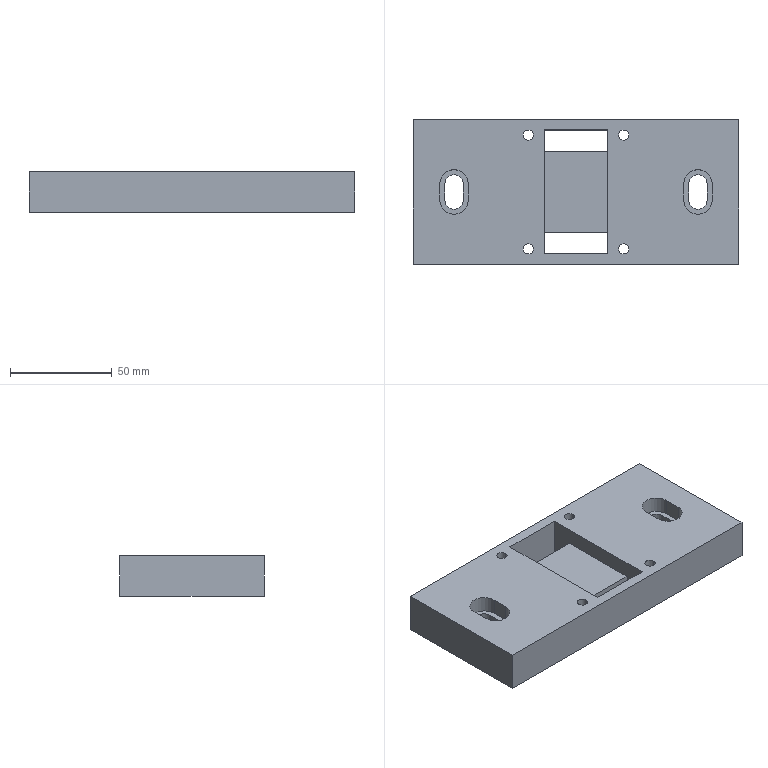Part | 1 solid | 39 faces | box 160 x 71 x 20 mm | volume 195179 mm3 | plane 23 | cylinder 16 | commonest cylinder face diameters 5 x8 9 x4 14 x4
STEP:
#1=CARTESIAN_POINT('',(-21.,28.,20.));
#2=VERTEX_POINT('',#1);
#3=CARTESIAN_POINT('',(-26.,28.,20.));
#4=VERTEX_POINT('',#3);
#5=CARTESIAN_POINT('',(-23.5,28.,20.));
#6=DIRECTION('',(0.,0.,-1.));
#7=DIRECTION('',(-1.,0.,0.));
#8=AXIS2_PLACEMENT_3D('',#5,#6,#7);
#9=CIRCLE('',#8,2.5);
#10=EDGE_CURVE('',#2,#4,#9,.T.);
#11=ORIENTED_EDGE('',*,*,#10,.F.);
#12=CARTESIAN_POINT('',(-21.,28.,0.));
#13=VERTEX_POINT('',#12);
#14=CARTESIAN_POINT('',(-21.,28.,0.));
#15=DIRECTION('',(0.,0.,-1.));
#16=VECTOR('',#15,1000.);
#17=LINE('',#14,#16);
#18=EDGE_CURVE('',#2,#13,#17,.T.);
#19=ORIENTED_EDGE('',*,*,#18,.T.);
#20=CARTESIAN_POINT('',(-26.,28.,0.));
#21=VERTEX_POINT('',#20);
#22=CARTESIAN_POINT('',(-23.5,28.,0.));
#23=DIRECTION('',(0.,0.,-1.));
#24=DIRECTION('',(-1.,0.,0.));
#25=AXIS2_PLACEMENT_3D('',#22,#23,#24);
#26=CIRCLE('',#25,2.5);
#27=EDGE_CURVE('',#13,#21,#26,.T.);
#28=ORIENTED_EDGE('',*,*,#27,.T.);
#29=CARTESIAN_POINT('',(-26.,28.,0.));
#30=DIRECTION('',(0.,0.,-1.));
#31=VECTOR('',#30,1000.);
#32=LINE('',#29,#31);
#33=EDGE_CURVE('',#4,#21,#32,.T.);
#34=ORIENTED_EDGE('',*,*,#33,.F.);
#35=EDGE_LOOP('',(#11,#19,#28,#34));
#36=FACE_OUTER_BOUND('',#35,.T.);
#37=CARTESIAN_POINT('',(-23.5,28.,0.));
#38=DIRECTION('',(0.,0.,-1.));
#39=DIRECTION('',(-1.,0.,0.));
#40=AXIS2_PLACEMENT_3D('',#37,#38,#39);
#41=CYLINDRICAL_SURFACE('',#40,2.5);
#42=ADVANCED_FACE('',(#36),#41,.F.);
#43=CARTESIAN_POINT('',(-21.,-28.,20.));
#44=VERTEX_POINT('',#43);
#45=CARTESIAN_POINT('',(-26.,-28.,20.));
#46=VERTEX_POINT('',#45);
#47=CARTESIAN_POINT('',(-23.5,-28.,20.));
#48=DIRECTION('',(0.,0.,-1.));
#49=DIRECTION('',(-1.,0.,0.));
#50=AXIS2_PLACEMENT_3D('',#47,#48,#49);
#51=CIRCLE('',#50,2.5);
#52=EDGE_CURVE('',#44,#46,#51,.T.);
#53=ORIENTED_EDGE('',*,*,#52,.F.);
#54=CARTESIAN_POINT('',(-21.,-28.,0.));
#55=VERTEX_POINT('',#54);
#56=CARTESIAN_POINT('',(-21.,-28.,0.));
#57=DIRECTION('',(0.,0.,-1.));
#58=VECTOR('',#57,1000.);
#59=LINE('',#56,#58);
#60=EDGE_CURVE('',#44,#55,#59,.T.);
#61=ORIENTED_EDGE('',*,*,#60,.T.);
#62=CARTESIAN_POINT('',(-26.,-28.,0.));
#63=VERTEX_POINT('',#62);
#64=CARTESIAN_POINT('',(-23.5,-28.,0.));
#65=DIRECTION('',(0.,0.,-1.));
#66=DIRECTION('',(-1.,0.,0.));
#67=AXIS2_PLACEMENT_3D('',#64,#65,#66);
#68=CIRCLE('',#67,2.5);
#69=EDGE_CURVE('',#55,#63,#68,.T.);
#70=ORIENTED_EDGE('',*,*,#69,.T.);
#71=CARTESIAN_POINT('',(-26.,-28.,0.));
#72=DIRECTION('',(0.,0.,-1.));
#73=VECTOR('',#72,1000.);
#74=LINE('',#71,#73);
#75=EDGE_CURVE('',#46,#63,#74,.T.);
#76=ORIENTED_EDGE('',*,*,#75,.F.);
#77=EDGE_LOOP('',(#53,#61,#70,#76));
#78=FACE_OUTER_BOUND('',#77,.T.);
#79=CARTESIAN_POINT('',(-23.5,-28.,0.));
#80=DIRECTION('',(0.,0.,-1.));
#81=DIRECTION('',(-1.,0.,0.));
#82=AXIS2_PLACEMENT_3D('',#79,#80,#81);
#83=CYLINDRICAL_SURFACE('',#82,2.5);
#84=ADVANCED_FACE('',(#78),#83,.F.);
#85=CARTESIAN_POINT('',(26.,-28.,20.));
#86=VERTEX_POINT('',#85);
#87=CARTESIAN_POINT('',(21.,-28.,20.));
#88=VERTEX_POINT('',#87);
#89=CARTESIAN_POINT('',(23.5,-28.,20.));
#90=DIRECTION('',(0.,0.,-1.));
#91=DIRECTION('',(-1.,0.,0.));
#92=AXIS2_PLACEMENT_3D('',#89,#90,#91);
#93=CIRCLE('',#92,2.5);
#94=EDGE_CURVE('',#86,#88,#93,.T.);
#95=ORIENTED_EDGE('',*,*,#94,.F.);
#96=CARTESIAN_POINT('',(26.,-28.,0.));
#97=VERTEX_POINT('',#96);
#98=CARTESIAN_POINT('',(26.,-28.,0.));
#99=DIRECTION('',(0.,0.,-1.));
#100=VECTOR('',#99,1000.);
#101=LINE('',#98,#100);
#102=EDGE_CURVE('',#86,#97,#101,.T.);
#103=ORIENTED_EDGE('',*,*,#102,.T.);
#104=CARTESIAN_POINT('',(21.,-28.,0.));
#105=VERTEX_POINT('',#104);
#106=CARTESIAN_POINT('',(23.5,-28.,0.));
#107=DIRECTION('',(0.,0.,-1.));
#108=DIRECTION('',(-1.,0.,0.));
#109=AXIS2_PLACEMENT_3D('',#106,#107,#108);
#110=CIRCLE('',#109,2.5);
#111=EDGE_CURVE('',#97,#105,#110,.T.);
#112=ORIENTED_EDGE('',*,*,#111,.T.);
#113=CARTESIAN_POINT('',(21.,-28.,0.));
#114=DIRECTION('',(0.,0.,-1.));
#115=VECTOR('',#114,1000.);
#116=LINE('',#113,#115);
#117=EDGE_CURVE('',#88,#105,#116,.T.);
#118=ORIENTED_EDGE('',*,*,#117,.F.);
#119=EDGE_LOOP('',(#95,#103,#112,#118));
#120=FACE_OUTER_BOUND('',#119,.T.);
#121=CARTESIAN_POINT('',(23.5,-28.,0.));
#122=DIRECTION('',(0.,0.,-1.));
#123=DIRECTION('',(-1.,0.,0.));
#124=AXIS2_PLACEMENT_3D('',#121,#122,#123);
#125=CYLINDRICAL_SURFACE('',#124,2.5);
#126=ADVANCED_FACE('',(#120),#125,.F.);
#127=CARTESIAN_POINT('',(26.,28.,20.));
#128=VERTEX_POINT('',#127);
#129=CARTESIAN_POINT('',(21.,28.,20.));
#130=VERTEX_POINT('',#129);
#131=CARTESIAN_POINT('',(23.5,28.,20.));
#132=DIRECTION('',(0.,0.,-1.));
#133=DIRECTION('',(-1.,0.,0.));
#134=AXIS2_PLACEMENT_3D('',#131,#132,#133);
#135=CIRCLE('',#134,2.5);
#136=EDGE_CURVE('',#128,#130,#135,.T.);
#137=ORIENTED_EDGE('',*,*,#136,.F.);
#138=CARTESIAN_POINT('',(26.,28.,0.));
#139=VERTEX_POINT('',#138);
#140=CARTESIAN_POINT('',(26.,28.,0.));
#141=DIRECTION('',(0.,0.,-1.));
#142=VECTOR('',#141,1000.);
#143=LINE('',#140,#142);
#144=EDGE_CURVE('',#128,#139,#143,.T.);
#145=ORIENTED_EDGE('',*,*,#144,.T.);
#146=CARTESIAN_POINT('',(21.,28.,0.));
#147=VERTEX_POINT('',#146);
#148=CARTESIAN_POINT('',(23.5,28.,0.));
#149=DIRECTION('',(0.,0.,-1.));
#150=DIRECTION('',(-1.,0.,0.));
#151=AXIS2_PLACEMENT_3D('',#148,#149,#150);
#152=CIRCLE('',#151,2.5);
#153=EDGE_CURVE('',#139,#147,#152,.T.);
#154=ORIENTED_EDGE('',*,*,#153,.T.);
#155=CARTESIAN_POINT('',(21.,28.,0.));
#156=DIRECTION('',(0.,0.,-1.));
#157=VECTOR('',#156,1000.);
#158=LINE('',#155,#157);
#159=EDGE_CURVE('',#130,#147,#158,.T.);
#160=ORIENTED_EDGE('',*,*,#159,.F.);
#161=EDGE_LOOP('',(#137,#145,#154,#160));
#162=FACE_OUTER_BOUND('',#161,.T.);
#163=CARTESIAN_POINT('',(23.5,28.,0.));
#164=DIRECTION('',(0.,0.,-1.));
#165=DIRECTION('',(-1.,0.,0.));
#166=AXIS2_PLACEMENT_3D('',#163,#164,#165);
#167=CYLINDRICAL_SURFACE('',#166,2.5);
#168=ADVANCED_FACE('',(#162),#167,.F.);
#169=CARTESIAN_POINT('',(-15.5,-30.5,20.));
#170=VERTEX_POINT('',#169);
#171=CARTESIAN_POINT('',(-15.5,-30.5,0.));
#172=VERTEX_POINT('',#171);
#173=CARTESIAN_POINT('',(-15.5,-30.5,20.));
#174=DIRECTION('',(0.,0.,-1.));
#175=VECTOR('',#174,1000.);
#176=LINE('',#173,#175);
#177=EDGE_CURVE('',#170,#172,#176,.T.);
#178=ORIENTED_EDGE('',*,*,#177,.T.);
#179=CARTESIAN_POINT('',(-15.5,-20.,0.));
#180=VERTEX_POINT('',#179);
#181=CARTESIAN_POINT('',(-15.5,-35.5,0.));
#182=DIRECTION('',(0.,1.,0.));
#183=VECTOR('',#182,1000.);
#184=LINE('',#181,#183);
#185=EDGE_CURVE('',#172,#180,#184,.T.);
#186=ORIENTED_EDGE('',*,*,#185,.T.);
#187=CARTESIAN_POINT('',(-15.5,-20.,12.));
#188=VERTEX_POINT('',#187);
#189=CARTESIAN_POINT('',(-15.5,-20.,-31.674));
#190=DIRECTION('',(0.,0.,1.));
#191=VECTOR('',#190,1000.);
#192=LINE('',#189,#191);
#193=EDGE_CURVE('',#180,#188,#192,.T.);
#194=ORIENTED_EDGE('',*,*,#193,.T.);
#195=CARTESIAN_POINT('',(-15.5,20.,12.));
#196=VERTEX_POINT('',#195);
#197=CARTESIAN_POINT('',(-15.5,-25.5,12.));
#198=DIRECTION('',(0.,1.,0.));
#199=VECTOR('',#198,1000.);
#200=LINE('',#197,#199);
#201=EDGE_CURVE('',#188,#196,#200,.T.);
#202=ORIENTED_EDGE('',*,*,#201,.T.);
#203=CARTESIAN_POINT('',(-15.5,20.,0.));
#204=VERTEX_POINT('',#203);
#205=CARTESIAN_POINT('',(-15.5,20.,-31.674));
#206=DIRECTION('',(0.,0.,1.));
#207=VECTOR('',#206,1000.);
#208=LINE('',#205,#207);
#209=EDGE_CURVE('',#204,#196,#208,.T.);
#210=ORIENTED_EDGE('',*,*,#209,.F.);
#211=CARTESIAN_POINT('',(-15.5,30.5,0.));
#212=VERTEX_POINT('',#211);
#213=CARTESIAN_POINT('',(-15.5,35.5,0.));
#214=DIRECTION('',(0.,-1.,0.));
#215=VECTOR('',#214,1000.);
#216=LINE('',#213,#215);
#217=EDGE_CURVE('',#212,#204,#216,.T.);
#218=ORIENTED_EDGE('',*,*,#217,.F.);
#219=CARTESIAN_POINT('',(-15.5,30.5,20.));
#220=VERTEX_POINT('',#219);
#221=CARTESIAN_POINT('',(-15.5,30.5,0.));
#222=DIRECTION('',(0.,0.,1.));
#223=VECTOR('',#222,1000.);
#224=LINE('',#221,#223);
#225=EDGE_CURVE('',#212,#220,#224,.T.);
#226=ORIENTED_EDGE('',*,*,#225,.T.);
#227=CARTESIAN_POINT('',(-15.5,35.5,20.));
#228=DIRECTION('',(0.,-1.,0.));
#229=VECTOR('',#228,1000.);
#230=LINE('',#227,#229);
#231=EDGE_CURVE('',#220,#170,#230,.T.);
#232=ORIENTED_EDGE('',*,*,#231,.T.);
#233=EDGE_LOOP('',(#178,#186,#194,#202,#210,#218,#226,#232));
#234=FACE_OUTER_BOUND('',#233,.T.);
#235=CARTESIAN_POINT('',(-15.5,35.5,0.));
#236=DIRECTION('',(-1.,0.,0.));
#237=DIRECTION('',(0.,-1.,0.));
#238=AXIS2_PLACEMENT_3D('',#235,#236,#237);
#239=PLANE('',#238);
#240=ADVANCED_FACE('',(#234),#239,.F.);
#241=CARTESIAN_POINT('',(15.5,-30.5,0.));
#242=VERTEX_POINT('',#241);
#243=CARTESIAN_POINT('',(15.5,-30.5,20.));
#244=VERTEX_POINT('',#243);
#245=CARTESIAN_POINT('',(15.5,-30.5,20.));
#246=DIRECTION('',(0.,0.,1.));
#247=VECTOR('',#246,1000.);
#248=LINE('',#245,#247);
#249=EDGE_CURVE('',#242,#244,#248,.T.);
#250=ORIENTED_EDGE('',*,*,#249,.T.);
#251=CARTESIAN_POINT('',(15.5,30.5,20.));
#252=VERTEX_POINT('',#251);
#253=CARTESIAN_POINT('',(15.5,35.5,20.));
#254=DIRECTION('',(0.,1.,0.));
#255=VECTOR('',#254,1000.);
#256=LINE('',#253,#255);
#257=EDGE_CURVE('',#244,#252,#256,.T.);
#258=ORIENTED_EDGE('',*,*,#257,.T.);
#259=CARTESIAN_POINT('',(15.5,30.5,0.));
#260=VERTEX_POINT('',#259);
#261=CARTESIAN_POINT('',(15.5,30.5,0.));
#262=DIRECTION('',(0.,0.,-1.));
#263=VECTOR('',#262,1000.);
#264=LINE('',#261,#263);
#265=EDGE_CURVE('',#252,#260,#264,.T.);
#266=ORIENTED_EDGE('',*,*,#265,.T.);
#267=CARTESIAN_POINT('',(15.5,20.,0.));
#268=VERTEX_POINT('',#267);
#269=CARTESIAN_POINT('',(15.5,35.5,0.));
#270=DIRECTION('',(0.,1.,0.));
#271=VECTOR('',#270,1000.);
#272=LINE('',#269,#271);
#273=EDGE_CURVE('',#268,#260,#272,.T.);
#274=ORIENTED_EDGE('',*,*,#273,.F.);
#275=CARTESIAN_POINT('',(15.5,20.,12.));
#276=VERTEX_POINT('',#275);
#277=CARTESIAN_POINT('',(15.5,20.,-31.674));
#278=DIRECTION('',(0.,0.,1.));
#279=VECTOR('',#278,1000.);
#280=LINE('',#277,#279);
#281=EDGE_CURVE('',#268,#276,#280,.T.);
#282=ORIENTED_EDGE('',*,*,#281,.T.);
#283=CARTESIAN_POINT('',(15.5,-20.,12.));
#284=VERTEX_POINT('',#283);
#285=CARTESIAN_POINT('',(15.5,-25.5,12.));
#286=DIRECTION('',(0.,1.,0.));
#287=VECTOR('',#286,1000.);
#288=LINE('',#285,#287);
#289=EDGE_CURVE('',#284,#276,#288,.T.);
#290=ORIENTED_EDGE('',*,*,#289,.F.);
#291=CARTESIAN_POINT('',(15.5,-20.,0.));
#292=VERTEX_POINT('',#291);
#293=CARTESIAN_POINT('',(15.5,-20.,-31.674));
#294=DIRECTION('',(0.,0.,1.));
#295=VECTOR('',#294,1000.);
#296=LINE('',#293,#295);
#297=EDGE_CURVE('',#292,#284,#296,.T.);
#298=ORIENTED_EDGE('',*,*,#297,.F.);
#299=CARTESIAN_POINT('',(15.5,-35.5,0.));
#300=DIRECTION('',(0.,-1.,0.));
#301=VECTOR('',#300,1000.);
#302=LINE('',#299,#301);
#303=EDGE_CURVE('',#292,#242,#302,.T.);
#304=ORIENTED_EDGE('',*,*,#303,.T.);
#305=EDGE_LOOP('',(#250,#258,#266,#274,#282,#290,#298,#304));
#306=FACE_OUTER_BOUND('',#305,.T.);
#307=CARTESIAN_POINT('',(15.5,35.5,0.));
#308=DIRECTION('',(1.,0.,0.));
#309=DIRECTION('',(0.,0.,-1.));
#310=AXIS2_PLACEMENT_3D('',#307,#308,#309);
#311=PLANE('',#310);
#312=ADVANCED_FACE('',(#306),#311,.F.);
#313=CARTESIAN_POINT('',(55.5,4.,12.));
#314=VERTEX_POINT('',#313);
#315=CARTESIAN_POINT('',(64.5,4.,12.));
#316=VERTEX_POINT('',#315);
#317=CARTESIAN_POINT('',(60.,4.,12.));
#318=DIRECTION('',(0.,0.,-1.));
#319=DIRECTION('',(1.,0.,0.));
#320=AXIS2_PLACEMENT_3D('',#317,#318,#319);
#321=CIRCLE('',#320,4.5);
#322=EDGE_CURVE('',#314,#316,#321,.T.);
#323=ORIENTED_EDGE('',*,*,#322,.F.);
#324=CARTESIAN_POINT('',(55.5,4.,0.));
#325=VERTEX_POINT('',#324);
#326=CARTESIAN_POINT('',(55.5,4.,20.));
#327=DIRECTION('',(0.,0.,-1.));
#328=VECTOR('',#327,1000.);
#329=LINE('',#326,#328);
#330=EDGE_CURVE('',#314,#325,#329,.T.);
#331=ORIENTED_EDGE('',*,*,#330,.T.);
#332=CARTESIAN_POINT('',(64.5,4.,0.));
#333=VERTEX_POINT('',#332);
#334=CARTESIAN_POINT('',(60.,4.,0.));
#335=DIRECTION('',(0.,0.,-1.));
#336=DIRECTION('',(-1.,0.,0.));
#337=AXIS2_PLACEMENT_3D('',#334,#335,#336);
#338=CIRCLE('',#337,4.5);
#339=EDGE_CURVE('',#325,#333,#338,.T.);
#340=ORIENTED_EDGE('',*,*,#339,.T.);
#341=CARTESIAN_POINT('',(64.5,4.,20.));
#342=DIRECTION('',(0.,0.,-1.));
#343=VECTOR('',#342,1000.);
#344=LINE('',#341,#343);
#345=EDGE_CURVE('',#316,#333,#344,.T.);
#346=ORIENTED_EDGE('',*,*,#345,.F.);
#347=EDGE_LOOP('',(#323,#331,#340,#346));
#348=FACE_OUTER_BOUND('',#347,.T.);
#349=CARTESIAN_POINT('',(60.,4.,20.));
#350=DIRECTION('',(0.,0.,-1.));
#351=DIRECTION('',(-1.,0.,0.));
#352=AXIS2_PLACEMENT_3D('',#349,#350,#351);
#353=CYLINDRICAL_SURFACE('',#352,4.5);
#354=ADVANCED_FACE('',(#348),#353,.F.);
#355=CARTESIAN_POINT('',(55.5,-4.,12.));
#356=VERTEX_POINT('',#355);
#357=CARTESIAN_POINT('',(55.5,4.,12.));
#358=DIRECTION('',(0.,1.,0.));
#359=VECTOR('',#358,1000.);
#360=LINE('',#357,#359);
#361=EDGE_CURVE('',#356,#314,#360,.T.);
#362=ORIENTED_EDGE('',*,*,#361,.F.);
#363=CARTESIAN_POINT('',(55.5,-4.,0.));
#364=VERTEX_POINT('',#363);
#365=CARTESIAN_POINT('',(55.5,-4.,20.));
#366=DIRECTION('',(0.,0.,-1.));
#367=VECTOR('',#366,1000.);
#368=LINE('',#365,#367);
#369=EDGE_CURVE('',#356,#364,#368,.T.);
#370=ORIENTED_EDGE('',*,*,#369,.T.);
#371=CARTESIAN_POINT('',(55.5,4.,0.));
#372=DIRECTION('',(0.,1.,0.));
#373=VECTOR('',#372,1000.);
#374=LINE('',#371,#373);
#375=EDGE_CURVE('',#364,#325,#374,.T.);
#376=ORIENTED_EDGE('',*,*,#375,.T.);
#377=ORIENTED_EDGE('',*,*,#330,.F.);
#378=EDGE_LOOP('',(#362,#370,#376,#377));
#379=FACE_OUTER_BOUND('',#378,.T.);
#380=CARTESIAN_POINT('',(55.5,4.,20.));
#381=DIRECTION('',(-1.,0.,0.));
#382=DIRECTION('',(0.,0.,1.));
#383=AXIS2_PLACEMENT_3D('',#380,#381,#382);
#384=PLANE('',#383);
#385=ADVANCED_FACE('',(#379),#384,.F.);
#386=CARTESIAN_POINT('',(64.5,-4.,12.));
#387=VERTEX_POINT('',#386);
#388=CARTESIAN_POINT('',(60.,-4.,12.));
#389=DIRECTION('',(0.,0.,-1.));
#390=DIRECTION('',(1.,0.,0.));
#391=AXIS2_PLACEMENT_3D('',#388,#389,#390);
#392=CIRCLE('',#391,4.5);
#393=EDGE_CURVE('',#387,#356,#392,.T.);
#394=ORIENTED_EDGE('',*,*,#393,.F.);
#395=CARTESIAN_POINT('',(64.5,-4.,0.));
#396=VERTEX_POINT('',#395);
#397=CARTESIAN_POINT('',(64.5,-4.,20.));
#398=DIRECTION('',(0.,0.,-1.));
#399=VECTOR('',#398,1000.);
#400=LINE('',#397,#399);
#401=EDGE_CURVE('',#387,#396,#400,.T.);
#402=ORIENTED_EDGE('',*,*,#401,.T.);
#403=CARTESIAN_POINT('',(60.,-4.,0.));
#404=DIRECTION('',(0.,0.,-1.));
#405=DIRECTION('',(-1.,0.,0.));
#406=AXIS2_PLACEMENT_3D('',#403,#404,#405);
#407=CIRCLE('',#406,4.5);
#408=EDGE_CURVE('',#396,#364,#407,.T.);
#409=ORIENTED_EDGE('',*,*,#408,.T.);
#410=ORIENTED_EDGE('',*,*,#369,.F.);
#411=EDGE_LOOP('',(#394,#402,#409,#410));
#412=FACE_OUTER_BOUND('',#411,.T.);
#413=CARTESIAN_POINT('',(60.,-4.,20.));
#414=DIRECTION('',(0.,0.,-1.));
#415=DIRECTION('',(-1.,0.,0.));
#416=AXIS2_PLACEMENT_3D('',#413,#414,#415);
#417=CYLINDRICAL_SURFACE('',#416,4.5);
#418=ADVANCED_FACE('',(#412),#417,.F.);
#419=CARTESIAN_POINT('',(64.5,4.,12.));
#420=DIRECTION('',(0.,-1.,0.));
#421=VECTOR('',#420,1000.);
#422=LINE('',#419,#421);
#423=EDGE_CURVE('',#316,#387,#422,.T.);
#424=ORIENTED_EDGE('',*,*,#423,.F.);
#425=ORIENTED_EDGE('',*,*,#345,.T.);
#426=CARTESIAN_POINT('',(64.5,4.,0.));
#427=DIRECTION('',(0.,-1.,0.));
#428=VECTOR('',#427,1000.);
#429=LINE('',#426,#428);
#430=EDGE_CURVE('',#333,#396,#429,.T.);
#431=ORIENTED_EDGE('',*,*,#430,.T.);
#432=ORIENTED_EDGE('',*,*,#401,.F.);
#433=EDGE_LOOP('',(#424,#425,#431,#432));
#434=FACE_OUTER_BOUND('',#433,.T.);
#435=CARTESIAN_POINT('',(64.5,4.,20.));
#436=DIRECTION('',(1.,0.,0.));
#437=DIRECTION('',(0.,0.,-1.));
#438=AXIS2_PLACEMENT_3D('',#435,#436,#437);
#439=PLANE('',#438);
#440=ADVANCED_FACE('',(#434),#439,.F.);
#441=CARTESIAN_POINT('',(-64.5,4.,12.));
#442=VERTEX_POINT('',#441);
#443=CARTESIAN_POINT('',(-55.5,4.,12.));
#444=VERTEX_POINT('',#443);
#445=CARTESIAN_POINT('',(-60.,4.,12.));
#446=DIRECTION('',(0.,0.,-1.));
#447=DIRECTION('',(1.,0.,0.));
#448=AXIS2_PLACEMENT_3D('',#445,#446,#447);
#449=CIRCLE('',#448,4.5);
#450=EDGE_CURVE('',#442,#444,#449,.T.);
#451=ORIENTED_EDGE('',*,*,#450,.F.);
#452=CARTESIAN_POINT('',(-64.5,4.,0.));
#453=VERTEX_POINT('',#452);
#454=CARTESIAN_POINT('',(-64.5,4.,20.));
#455=DIRECTION('',(0.,0.,-1.));
#456=VECTOR('',#455,1000.);
#457=LINE('',#454,#456);
#458=EDGE_CURVE('',#442,#453,#457,.T.);
#459=ORIENTED_EDGE('',*,*,#458,.T.);
#460=CARTESIAN_POINT('',(-55.5,4.,0.));
#461=VERTEX_POINT('',#460);
#462=CARTESIAN_POINT('',(-60.,4.,0.));
#463=DIRECTION('',(0.,0.,-1.));
#464=DIRECTION('',(-1.,0.,0.));
#465=AXIS2_PLACEMENT_3D('',#462,#463,#464);
#466=CIRCLE('',#465,4.5);
#467=EDGE_CURVE('',#453,#461,#466,.T.);
#468=ORIENTED_EDGE('',*,*,#467,.T.);
#469=CARTESIAN_POINT('',(-55.5,4.,20.));
#470=DIRECTION('',(0.,0.,-1.));
#471=VECTOR('',#470,1000.);
#472=LINE('',#469,#471);
#473=EDGE_CURVE('',#444,#461,#472,.T.);
#474=ORIENTED_EDGE('',*,*,#473,.F.);
#475=EDGE_LOOP('',(#451,#459,#468,#474));
#476=FACE_OUTER_BOUND('',#475,.T.);
#477=CARTESIAN_POINT('',(-60.,4.,20.));
#478=DIRECTION('',(0.,0.,-1.));
#479=DIRECTION('',(-1.,0.,0.));
#480=AXIS2_PLACEMENT_3D('',#477,#478,#479);
#481=CYLINDRICAL_SURFACE('',#480,4.5);
#482=ADVANCED_FACE('',(#476),#481,.F.);
#483=CARTESIAN_POINT('',(-64.5,-4.,12.));
#484=VERTEX_POINT('',#483);
#485=CARTESIAN_POINT('',(-64.5,4.,12.));
#486=DIRECTION('',(0.,1.,0.));
#487=VECTOR('',#486,1000.);
#488=LINE('',#485,#487);
#489=EDGE_CURVE('',#484,#442,#488,.T.);
#490=ORIENTED_EDGE('',*,*,#489,.F.);
#491=CARTESIAN_POINT('',(-64.5,-4.,0.));
#492=VERTEX_POINT('',#491);
#493=CARTESIAN_POINT('',(-64.5,-4.,20.));
#494=DIRECTION('',(0.,0.,-1.));
#495=VECTOR('',#494,1000.);
#496=LINE('',#493,#495);
#497=EDGE_CURVE('',#484,#492,#496,.T.);
#498=ORIENTED_EDGE('',*,*,#497,.T.);
#499=CARTESIAN_POINT('',(-64.5,4.,0.));
#500=DIRECTION('',(0.,1.,0.));
#501=VECTOR('',#500,1000.);
#502=LINE('',#499,#501);
#503=EDGE_CURVE('',#492,#453,#502,.T.);
#504=ORIENTED_EDGE('',*,*,#503,.T.);
#505=ORIENTED_EDGE('',*,*,#458,.F.);
#506=EDGE_LOOP('',(#490,#498,#504,#505));
#507=FACE_OUTER_BOUND('',#506,.T.);
#508=CARTESIAN_POINT('',(-64.5,4.,20.));
#509=DIRECTION('',(-1.,0.,0.));
#510=DIRECTION('',(0.,0.,1.));
#511=AXIS2_PLACEMENT_3D('',#508,#509,#510);
#512=PLANE('',#511);
#513=ADVANCED_FACE('',(#507),#512,.F.);
#514=CARTESIAN_POINT('',(-55.5,-4.,12.));
#515=VERTEX_POINT('',#514);
#516=CARTESIAN_POINT('',(-60.,-4.,12.));
#517=DIRECTION('',(0.,0.,-1.));
#518=DIRECTION('',(1.,0.,0.));
#519=AXIS2_PLACEMENT_3D('',#516,#517,#518);
#520=CIRCLE('',#519,4.5);
#521=EDGE_CURVE('',#515,#484,#520,.T.);
#522=ORIENTED_EDGE('',*,*,#521,.F.);
#523=CARTESIAN_POINT('',(-55.5,-4.,0.));
#524=VERTEX_POINT('',#523);
#525=CARTESIAN_POINT('',(-55.5,-4.,20.));
#526=DIRECTION('',(0.,0.,-1.));
#527=VECTOR('',#526,1000.);
#528=LINE('',#525,#527);
#529=EDGE_CURVE('',#515,#524,#528,.T.);
#530=ORIENTED_EDGE('',*,*,#529,.T.);
#531=CARTESIAN_POINT('',(-60.,-4.,0.));
#532=DIRECTION('',(0.,0.,-1.));
#533=DIRECTION('',(-1.,0.,0.));
#534=AXIS2_PLACEMENT_3D('',#531,#532,#533);
#535=CIRCLE('',#534,4.5);
#536=EDGE_CURVE('',#524,#492,#535,.T.);
#537=ORIENTED_EDGE('',*,*,#536,.T.);
#538=ORIENTED_EDGE('',*,*,#497,.F.);
#539=EDGE_LOOP('',(#522,#530,#537,#538));
#540=FACE_OUTER_BOUND('',#539,.T.);
#541=CARTESIAN_POINT('',(-60.,-4.,20.));
#542=DIRECTION('',(0.,0.,-1.));
#543=DIRECTION('',(-1.,0.,0.));
#544=AXIS2_PLACEMENT_3D('',#541,#542,#543);
#545=CYLINDRICAL_SURFACE('',#544,4.5);
#546=ADVANCED_FACE('',(#540),#545,.F.);
#547=CARTESIAN_POINT('',(-55.5,4.,12.));
#548=DIRECTION('',(0.,-1.,0.));
#549=VECTOR('',#548,1000.);
#550=LINE('',#547,#549);
#551=EDGE_CURVE('',#444,#515,#550,.T.);
#552=ORIENTED_EDGE('',*,*,#551,.F.);
#553=ORIENTED_EDGE('',*,*,#473,.T.);
#554=CARTESIAN_POINT('',(-55.5,4.,0.));
#555=DIRECTION('',(0.,-1.,0.));
#556=VECTOR('',#555,1000.);
#557=LINE('',#554,#556);
#558=EDGE_CURVE('',#461,#524,#557,.T.);
#559=ORIENTED_EDGE('',*,*,#558,.T.);
#560=ORIENTED_EDGE('',*,*,#529,.F.);
#561=EDGE_LOOP('',(#552,#553,#559,#560));
#562=FACE_OUTER_BOUND('',#561,.T.);
#563=CARTESIAN_POINT('',(-55.5,4.,20.));
#564=DIRECTION('',(1.,0.,0.));
#565=DIRECTION('',(0.,0.,-1.));
#566=AXIS2_PLACEMENT_3D('',#563,#564,#565);
#567=PLANE('',#566);
#568=ADVANCED_FACE('',(#562),#567,.F.);
#569=CARTESIAN_POINT('',(-80.,35.5,20.));
#570=VERTEX_POINT('',#569);
#571=CARTESIAN_POINT('',(-80.,-35.5,20.));
#572=VERTEX_POINT('',#571);
#573=CARTESIAN_POINT('',(-80.,-30.,20.));
#574=DIRECTION('',(0.,-1.,0.));
#575=VECTOR('',#574,1000.);
#576=LINE('',#573,#575);
#577=EDGE_CURVE('',#570,#572,#576,.T.);
#578=ORIENTED_EDGE('',*,*,#577,.T.);
#579=CARTESIAN_POINT('',(80.,-35.5,20.));
#580=VERTEX_POINT('',#579);
#581=CARTESIAN_POINT('',(80.,-35.5,20.));
#582=DIRECTION('',(-1.,0.,0.));
#583=VECTOR('',#582,1000.);
#584=LINE('',#581,#583);
#585=EDGE_CURVE('',#580,#572,#584,.T.);
#586=ORIENTED_EDGE('',*,*,#585,.F.);
#587=CARTESIAN_POINT('',(80.,35.5,20.));
#588=VERTEX_POINT('',#587);
#589=CARTESIAN_POINT('',(80.,-30.,20.));
#590=DIRECTION('',(0.,1.,0.));
#591=VECTOR('',#590,1000.);
#592=LINE('',#589,#591);
#593=EDGE_CURVE('',#580,#588,#592,.T.);
#594=ORIENTED_EDGE('',*,*,#593,.T.);
#595=CARTESIAN_POINT('',(-80.,35.5,20.));
#596=DIRECTION('',(1.,0.,0.));
#597=VECTOR('',#596,1000.);
#598=LINE('',#595,#597);
#599=EDGE_CURVE('',#570,#588,#598,.T.);
#600=ORIENTED_EDGE('',*,*,#599,.F.);
#601=EDGE_LOOP('',(#578,#586,#594,#600));
#602=FACE_OUTER_BOUND('',#601,.T.);
#603=CARTESIAN_POINT('',(53.,4.,20.));
#604=VERTEX_POINT('',#603);
#605=CARTESIAN_POINT('',(53.,-4.,20.));
#606=VERTEX_POINT('',#605);
#607=CARTESIAN_POINT('',(53.,4.,20.));
#608=DIRECTION('',(0.,-1.,0.));
#609=VECTOR('',#608,1000.);
#610=LINE('',#607,#609);
#611=EDGE_CURVE('',#604,#606,#610,.T.);
#612=ORIENTED_EDGE('',*,*,#611,.F.);
#613=CARTESIAN_POINT('',(67.,4.,20.));
#614=VERTEX_POINT('',#613);
#615=CARTESIAN_POINT('',(60.,4.,20.));
#616=DIRECTION('',(0.,0.,1.));
#617=DIRECTION('',(1.,0.,0.));
#618=AXIS2_PLACEMENT_3D('',#615,#616,#617);
#619=CIRCLE('',#618,7.);
#620=EDGE_CURVE('',#614,#604,#619,.T.);
#621=ORIENTED_EDGE('',*,*,#620,.F.);
#622=CARTESIAN_POINT('',(67.,-4.,20.));
#623=VERTEX_POINT('',#622);
#624=CARTESIAN_POINT('',(67.,4.,20.));
#625=DIRECTION('',(0.,1.,0.));
#626=VECTOR('',#625,1000.);
#627=LINE('',#624,#626);
#628=EDGE_CURVE('',#623,#614,#627,.T.);
#629=ORIENTED_EDGE('',*,*,#628,.F.);
#630=CARTESIAN_POINT('',(60.,-4.,20.));
#631=DIRECTION('',(0.,0.,1.));
#632=DIRECTION('',(1.,0.,0.));
#633=AXIS2_PLACEMENT_3D('',#630,#631,#632);
#634=CIRCLE('',#633,7.);
#635=EDGE_CURVE('',#606,#623,#634,.T.);
#636=ORIENTED_EDGE('',*,*,#635,.F.);
#637=EDGE_LOOP('',(#612,#621,#629,#636));
#638=FACE_BOUND('',#637,.T.);
#639=CARTESIAN_POINT('',(23.5,28.,20.));
#640=DIRECTION('',(0.,0.,-1.));
#641=DIRECTION('',(-1.,0.,0.));
#642=AXIS2_PLACEMENT_3D('',#639,#640,#641);
#643=CIRCLE('',#642,2.5);
#644=EDGE_CURVE('',#130,#128,#643,.T.);
#645=ORIENTED_EDGE('',*,*,#644,.T.);
#646=ORIENTED_EDGE('',*,*,#136,.T.);
#647=EDGE_LOOP('',(#645,#646));
#648=FACE_BOUND('',#647,.T.);
#649=CARTESIAN_POINT('',(23.5,-28.,20.));
#650=DIRECTION('',(0.,0.,-1.));
#651=DIRECTION('',(-1.,0.,0.));
#652=AXIS2_PLACEMENT_3D('',#649,#650,#651);
#653=CIRCLE('',#652,2.5);
#654=EDGE_CURVE('',#88,#86,#653,.T.);
#655=ORIENTED_EDGE('',*,*,#654,.T.);
#656=ORIENTED_EDGE('',*,*,#94,.T.);
#657=EDGE_LOOP('',(#655,#656));
#658=FACE_BOUND('',#657,.T.);
#659=ORIENTED_EDGE('',*,*,#257,.F.);
#660=CARTESIAN_POINT('',(-15.5,-30.5,20.));
#661=DIRECTION('',(-1.,0.,0.));
#662=VECTOR('',#661,1000.);
#663=LINE('',#660,#662);
#664=EDGE_CURVE('',#244,#170,#663,.T.);
#665=ORIENTED_EDGE('',*,*,#664,.T.);
#666=ORIENTED_EDGE('',*,*,#231,.F.);
#667=CARTESIAN_POINT('',(-15.5,30.5,20.));
#668=DIRECTION('',(1.,0.,0.));
#669=VECTOR('',#668,1000.);
#670=LINE('',#667,#669);
#671=EDGE_CURVE('',#220,#252,#670,.T.);
#672=ORIENTED_EDGE('',*,*,#671,.T.);
#673=EDGE_LOOP('',(#659,#665,#666,#672));
#674=FACE_BOUND('',#673,.T.);
#675=CARTESIAN_POINT('',(-67.,4.,20.));
#676=VERTEX_POINT('',#675);
#677=CARTESIAN_POINT('',(-67.,-4.,20.));
#678=VERTEX_POINT('',#677);
#679=CARTESIAN_POINT('',(-67.,4.,20.));
#680=DIRECTION('',(0.,-1.,0.));
#681=VECTOR('',#680,1000.);
#682=LINE('',#679,#681);
#683=EDGE_CURVE('',#676,#678,#682,.T.);
#684=ORIENTED_EDGE('',*,*,#683,.F.);
#685=CARTESIAN_POINT('',(-53.,4.,20.));
#686=VERTEX_POINT('',#685);
#687=CARTESIAN_POINT('',(-60.,4.,20.));
#688=DIRECTION('',(0.,0.,1.));
#689=DIRECTION('',(1.,0.,0.));
#690=AXIS2_PLACEMENT_3D('',#687,#688,#689);
#691=CIRCLE('',#690,7.);
#692=EDGE_CURVE('',#686,#676,#691,.T.);
#693=ORIENTED_EDGE('',*,*,#692,.F.);
#694=CARTESIAN_POINT('',(-53.,-4.,20.));
#695=VERTEX_POINT('',#694);
#696=CARTESIAN_POINT('',(-53.,4.,20.));
#697=DIRECTION('',(0.,1.,0.));
#698=VECTOR('',#697,1000.);
#699=LINE('',#696,#698);
#700=EDGE_CURVE('',#695,#686,#699,.T.);
#701=ORIENTED_EDGE('',*,*,#700,.F.);
#702=CARTESIAN_POINT('',(-60.,-4.,20.));
#703=DIRECTION('',(0.,0.,1.));
#704=DIRECTION('',(1.,0.,0.));
#705=AXIS2_PLACEMENT_3D('',#702,#703,#704);
#706=CIRCLE('',#705,7.);
#707=EDGE_CURVE('',#678,#695,#706,.T.);
#708=ORIENTED_EDGE('',*,*,#707,.F.);
#709=EDGE_LOOP('',(#684,#693,#701,#708));
#710=FACE_BOUND('',#709,.T.);
#711=CARTESIAN_POINT('',(-23.5,28.,20.));
#712=DIRECTION('',(0.,0.,-1.));
#713=DIRECTION('',(-1.,0.,0.));
#714=AXIS2_PLACEMENT_3D('',#711,#712,#713);
#715=CIRCLE('',#714,2.5);
#716=EDGE_CURVE('',#4,#2,#715,.T.);
#717=ORIENTED_EDGE('',*,*,#716,.T.);
#718=ORIENTED_EDGE('',*,*,#10,.T.);
#719=EDGE_LOOP('',(#717,#718));
#720=FACE_BOUND('',#719,.T.);
#721=CARTESIAN_POINT('',(-23.5,-28.,20.));
#722=DIRECTION('',(0.,0.,-1.));
#723=DIRECTION('',(-1.,0.,0.));
#724=AXIS2_PLACEMENT_3D('',#721,#722,#723);
#725=CIRCLE('',#724,2.5);
#726=EDGE_CURVE('',#46,#44,#725,.T.);
#727=ORIENTED_EDGE('',*,*,#726,.T.);
#728=ORIENTED_EDGE('',*,*,#52,.T.);
#729=EDGE_LOOP('',(#727,#728));
#730=FACE_BOUND('',#729,.T.);
#731=CARTESIAN_POINT('',(0.,0.,20.));
#732=DIRECTION('',(0.,0.,-1.));
#733=DIRECTION('',(-1.,0.,0.));
#734=AXIS2_PLACEMENT_3D('',#731,#732,#733);
#735=PLANE('',#734);
#736=ADVANCED_FACE('',(#602,#638,#648,#658,#674,#710,#720,#730),#735,.F.);
#737=ORIENTED_EDGE('',*,*,#185,.F.);
#738=CARTESIAN_POINT('',(-15.5,-30.5,0.));
#739=DIRECTION('',(1.,0.,0.));
#740=VECTOR('',#739,1000.);
#741=LINE('',#738,#740);
#742=EDGE_CURVE('',#172,#242,#741,.T.);
#743=ORIENTED_EDGE('',*,*,#742,.T.);
#744=ORIENTED_EDGE('',*,*,#303,.F.);
#745=CARTESIAN_POINT('',(-15.5,-20.,0.));
#746=DIRECTION('',(1.,0.,0.));
#747=VECTOR('',#746,1000.);
#748=LINE('',#745,#747);
#749=EDGE_CURVE('',#180,#292,#748,.T.);
#750=ORIENTED_EDGE('',*,*,#749,.F.);
#751=EDGE_LOOP('',(#737,#743,#744,#750));
#752=FACE_BOUND('',#751,.T.);
#753=CARTESIAN_POINT('',(-15.5,30.5,0.));
#754=DIRECTION('',(-1.,0.,0.));
#755=VECTOR('',#754,1000.);
#756=LINE('',#753,#755);
#757=EDGE_CURVE('',#260,#212,#756,.T.);
#758=ORIENTED_EDGE('',*,*,#757,.T.);
#759=ORIENTED_EDGE('',*,*,#217,.T.);
#760=CARTESIAN_POINT('',(-15.5,20.,0.));
#761=DIRECTION('',(-1.,0.,0.));
#762=VECTOR('',#761,1000.);
#763=LINE('',#760,#762);
#764=EDGE_CURVE('',#268,#204,#763,.T.);
#765=ORIENTED_EDGE('',*,*,#764,.F.);
#766=ORIENTED_EDGE('',*,*,#273,.T.);
#767=EDGE_LOOP('',(#758,#759,#765,#766));
#768=FACE_BOUND('',#767,.T.);
#769=CARTESIAN_POINT('',(80.,-35.5,0.));
#770=VERTEX_POINT('',#769);
#771=CARTESIAN_POINT('',(80.,35.5,0.));
#772=VERTEX_POINT('',#771);
#773=CARTESIAN_POINT('',(80.,-30.,0.));
#774=DIRECTION('',(0.,1.,0.));
#775=VECTOR('',#774,1000.);
#776=LINE('',#773,#775);
#777=EDGE_CURVE('',#770,#772,#776,.T.);
#778=ORIENTED_EDGE('',*,*,#777,.F.);
#779=CARTESIAN_POINT('',(-80.,-35.5,0.));
#780=VERTEX_POINT('',#779);
#781=CARTESIAN_POINT('',(-80.,-35.5,0.));
#782=DIRECTION('',(1.,0.,0.));
#783=VECTOR('',#782,1000.);
#784=LINE('',#781,#783);
#785=EDGE_CURVE('',#780,#770,#784,.T.);
#786=ORIENTED_EDGE('',*,*,#785,.F.);
#787=CARTESIAN_POINT('',(-80.,35.5,0.));
#788=VERTEX_POINT('',#787);
#789=CARTESIAN_POINT('',(-80.,-30.,0.));
#790=DIRECTION('',(0.,-1.,0.));
#791=VECTOR('',#790,1000.);
#792=LINE('',#789,#791);
#793=EDGE_CURVE('',#788,#780,#792,.T.);
#794=ORIENTED_EDGE('',*,*,#793,.F.);
#795=CARTESIAN_POINT('',(80.,35.5,0.));
#796=DIRECTION('',(-1.,0.,0.));
#797=VECTOR('',#796,1000.);
#798=LINE('',#795,#797);
#799=EDGE_CURVE('',#772,#788,#798,.T.);
#800=ORIENTED_EDGE('',*,*,#799,.F.);
#801=EDGE_LOOP('',(#778,#786,#794,#800));
#802=FACE_OUTER_BOUND('',#801,.T.);
#803=ORIENTED_EDGE('',*,*,#467,.F.);
#804=ORIENTED_EDGE('',*,*,#503,.F.);
#805=ORIENTED_EDGE('',*,*,#536,.F.);
#806=ORIENTED_EDGE('',*,*,#558,.F.);
#807=EDGE_LOOP('',(#803,#804,#805,#806));
#808=FACE_BOUND('',#807,.T.);
#809=ORIENTED_EDGE('',*,*,#339,.F.);
#810=ORIENTED_EDGE('',*,*,#375,.F.);
#811=ORIENTED_EDGE('',*,*,#408,.F.);
#812=ORIENTED_EDGE('',*,*,#430,.F.);
#813=EDGE_LOOP('',(#809,#810,#811,#812));
#814=FACE_BOUND('',#813,.T.);
#815=CARTESIAN_POINT('',(23.5,28.,0.));
#816=DIRECTION('',(0.,0.,-1.));
#817=DIRECTION('',(-1.,0.,0.));
#818=AXIS2_PLACEMENT_3D('',#815,#816,#817);
#819=CIRCLE('',#818,2.5);
#820=EDGE_CURVE('',#147,#139,#819,.T.);
#821=ORIENTED_EDGE('',*,*,#820,.F.);
#822=ORIENTED_EDGE('',*,*,#153,.F.);
#823=EDGE_LOOP('',(#821,#822));
#824=FACE_BOUND('',#823,.T.);
#825=CARTESIAN_POINT('',(23.5,-28.,0.));
#826=DIRECTION('',(0.,0.,-1.));
#827=DIRECTION('',(-1.,0.,0.));
#828=AXIS2_PLACEMENT_3D('',#825,#826,#827);
#829=CIRCLE('',#828,2.5);
#830=EDGE_CURVE('',#105,#97,#829,.T.);
#831=ORIENTED_EDGE('',*,*,#830,.F.);
#832=ORIENTED_EDGE('',*,*,#111,.F.);
#833=EDGE_LOOP('',(#831,#832));
#834=FACE_BOUND('',#833,.T.);
#835=CARTESIAN_POINT('',(-23.5,-28.,0.));
#836=DIRECTION('',(0.,0.,-1.));
#837=DIRECTION('',(-1.,0.,0.));
#838=AXIS2_PLACEMENT_3D('',#835,#836,#837);
#839=CIRCLE('',#838,2.5);
#840=EDGE_CURVE('',#63,#55,#839,.T.);
#841=ORIENTED_EDGE('',*,*,#840,.F.);
#842=ORIENTED_EDGE('',*,*,#69,.F.);
#843=EDGE_LOOP('',(#841,#842));
#844=FACE_BOUND('',#843,.T.);
#845=CARTESIAN_POINT('',(-23.5,28.,0.));
#846=DIRECTION('',(0.,0.,-1.));
#847=DIRECTION('',(-1.,0.,0.));
#848=AXIS2_PLACEMENT_3D('',#845,#846,#847);
#849=CIRCLE('',#848,2.5);
#850=EDGE_CURVE('',#21,#13,#849,.T.);
#851=ORIENTED_EDGE('',*,*,#850,.F.);
#852=ORIENTED_EDGE('',*,*,#27,.F.);
#853=EDGE_LOOP('',(#851,#852));
#854=FACE_BOUND('',#853,.T.);
#855=CARTESIAN_POINT('',(0.,0.,0.));
#856=DIRECTION('',(0.,0.,-1.));
#857=DIRECTION('',(-1.,0.,0.));
#858=AXIS2_PLACEMENT_3D('',#855,#856,#857);
#859=PLANE('',#858);
#860=ADVANCED_FACE('',(#752,#768,#802,#808,#814,#824,#834,#844,#854),#859,.T.);
#861=ORIENTED_EDGE('',*,*,#585,.T.);
#862=CARTESIAN_POINT('',(-80.,-35.5,20.));
#863=DIRECTION('',(0.,0.,-1.));
#864=VECTOR('',#863,1000.);
#865=LINE('',#862,#864);
#866=EDGE_CURVE('',#572,#780,#865,.T.);
#867=ORIENTED_EDGE('',*,*,#866,.T.);
#868=ORIENTED_EDGE('',*,*,#785,.T.);
#869=CARTESIAN_POINT('',(80.,-35.5,0.));
#870=DIRECTION('',(0.,0.,1.));
#871=VECTOR('',#870,1000.);
#872=LINE('',#869,#871);
#873=EDGE_CURVE('',#770,#580,#872,.T.);
#874=ORIENTED_EDGE('',*,*,#873,.T.);
#875=EDGE_LOOP('',(#861,#867,#868,#874));
#876=FACE_OUTER_BOUND('',#875,.T.);
#877=CARTESIAN_POINT('',(0.,-35.5,0.));
#878=DIRECTION('',(0.,-1.,0.));
#879=DIRECTION('',(0.,0.,-1.));
#880=AXIS2_PLACEMENT_3D('',#877,#878,#879);
#881=PLANE('',#880);
#882=ADVANCED_FACE('',(#876),#881,.T.);
#883=ORIENTED_EDGE('',*,*,#777,.T.);
#884=CARTESIAN_POINT('',(80.,35.5,20.));
#885=DIRECTION('',(0.,0.,-1.));
#886=VECTOR('',#885,1000.);
#887=LINE('',#884,#886);
#888=EDGE_CURVE('',#588,#772,#887,.T.);
#889=ORIENTED_EDGE('',*,*,#888,.F.);
#890=ORIENTED_EDGE('',*,*,#593,.F.);
#891=ORIENTED_EDGE('',*,*,#873,.F.);
#892=EDGE_LOOP('',(#883,#889,#890,#891));
#893=FACE_OUTER_BOUND('',#892,.T.);
#894=CARTESIAN_POINT('',(80.,-30.,20.));
#895=DIRECTION('',(-1.,0.,0.));
#896=DIRECTION('',(0.,0.,1.));
#897=AXIS2_PLACEMENT_3D('',#894,#895,#896);
#898=PLANE('',#897);
#899=ADVANCED_FACE('',(#893),#898,.F.);
#900=ORIENTED_EDGE('',*,*,#793,.T.);
#901=ORIENTED_EDGE('',*,*,#866,.F.);
#902=ORIENTED_EDGE('',*,*,#577,.F.);
#903=CARTESIAN_POINT('',(-80.,35.5,0.));
#904=DIRECTION('',(0.,0.,1.));
#905=VECTOR('',#904,1000.);
#906=LINE('',#903,#905);
#907=EDGE_CURVE('',#788,#570,#906,.T.);
#908=ORIENTED_EDGE('',*,*,#907,.F.);
#909=EDGE_LOOP('',(#900,#901,#902,#908));
#910=FACE_OUTER_BOUND('',#909,.T.);
#911=CARTESIAN_POINT('',(-80.,-30.,20.));
#912=DIRECTION('',(1.,0.,0.));
#913=DIRECTION('',(0.,0.,-1.));
#914=AXIS2_PLACEMENT_3D('',#911,#912,#913);
#915=PLANE('',#914);
#916=ADVANCED_FACE('',(#910),#915,.F.);
#917=ORIENTED_EDGE('',*,*,#799,.T.);
#918=ORIENTED_EDGE('',*,*,#907,.T.);
#919=ORIENTED_EDGE('',*,*,#599,.T.);
#920=ORIENTED_EDGE('',*,*,#888,.T.);
#921=EDGE_LOOP('',(#917,#918,#919,#920));
#922=FACE_OUTER_BOUND('',#921,.T.);
#923=CARTESIAN_POINT('',(0.,35.5,0.));
#924=DIRECTION('',(0.,1.,0.));
#925=DIRECTION('',(0.,0.,1.));
#926=AXIS2_PLACEMENT_3D('',#923,#924,#925);
#927=PLANE('',#926);
#928=ADVANCED_FACE('',(#922),#927,.T.);
#929=ORIENTED_EDGE('',*,*,#144,.F.);
#930=ORIENTED_EDGE('',*,*,#644,.F.);
#931=ORIENTED_EDGE('',*,*,#159,.T.);
#932=ORIENTED_EDGE('',*,*,#820,.T.);
#933=EDGE_LOOP('',(#929,#930,#931,#932));
#934=FACE_OUTER_BOUND('',#933,.T.);
#935=CARTESIAN_POINT('',(23.5,28.,0.));
#936=DIRECTION('',(0.,0.,-1.));
#937=DIRECTION('',(-1.,0.,0.));
#938=AXIS2_PLACEMENT_3D('',#935,#936,#937);
#939=CYLINDRICAL_SURFACE('',#938,2.5);
#940=ADVANCED_FACE('',(#934),#939,.F.);
#941=ORIENTED_EDGE('',*,*,#102,.F.);
#942=ORIENTED_EDGE('',*,*,#654,.F.);
#943=ORIENTED_EDGE('',*,*,#117,.T.);
#944=ORIENTED_EDGE('',*,*,#830,.T.);
#945=EDGE_LOOP('',(#941,#942,#943,#944));
#946=FACE_OUTER_BOUND('',#945,.T.);
#947=CARTESIAN_POINT('',(23.5,-28.,0.));
#948=DIRECTION('',(0.,0.,-1.));
#949=DIRECTION('',(-1.,0.,0.));
#950=AXIS2_PLACEMENT_3D('',#947,#948,#949);
#951=CYLINDRICAL_SURFACE('',#950,2.5);
#952=ADVANCED_FACE('',(#946),#951,.F.);
#953=ORIENTED_EDGE('',*,*,#60,.F.);
#954=ORIENTED_EDGE('',*,*,#726,.F.);
#955=ORIENTED_EDGE('',*,*,#75,.T.);
#956=ORIENTED_EDGE('',*,*,#840,.T.);
#957=EDGE_LOOP('',(#953,#954,#955,#956));
#958=FACE_OUTER_BOUND('',#957,.T.);
#959=CARTESIAN_POINT('',(-23.5,-28.,0.));
#960=DIRECTION('',(0.,0.,-1.));
#961=DIRECTION('',(-1.,0.,0.));
#962=AXIS2_PLACEMENT_3D('',#959,#960,#961);
#963=CYLINDRICAL_SURFACE('',#962,2.5);
#964=ADVANCED_FACE('',(#958),#963,.F.);
#965=ORIENTED_EDGE('',*,*,#18,.F.);
#966=ORIENTED_EDGE('',*,*,#716,.F.);
#967=ORIENTED_EDGE('',*,*,#33,.T.);
#968=ORIENTED_EDGE('',*,*,#850,.T.);
#969=EDGE_LOOP('',(#965,#966,#967,#968));
#970=FACE_OUTER_BOUND('',#969,.T.);
#971=CARTESIAN_POINT('',(-23.5,28.,0.));
#972=DIRECTION('',(0.,0.,-1.));
#973=DIRECTION('',(-1.,0.,0.));
#974=AXIS2_PLACEMENT_3D('',#971,#972,#973);
#975=CYLINDRICAL_SURFACE('',#974,2.5);
#976=ADVANCED_FACE('',(#970),#975,.F.);
#977=ORIENTED_EDGE('',*,*,#201,.F.);
#978=CARTESIAN_POINT('',(-15.5,-20.,12.));
#979=DIRECTION('',(1.,0.,0.));
#980=VECTOR('',#979,1000.);
#981=LINE('',#978,#980);
#982=EDGE_CURVE('',#188,#284,#981,.T.);
#983=ORIENTED_EDGE('',*,*,#982,.T.);
#984=ORIENTED_EDGE('',*,*,#289,.T.);
#985=CARTESIAN_POINT('',(-15.5,20.,12.));
#986=DIRECTION('',(-1.,0.,0.));
#987=VECTOR('',#986,1000.);
#988=LINE('',#985,#987);
#989=EDGE_CURVE('',#276,#196,#988,.T.);
#990=ORIENTED_EDGE('',*,*,#989,.T.);
#991=EDGE_LOOP('',(#977,#983,#984,#990));
#992=FACE_OUTER_BOUND('',#991,.T.);
#993=CARTESIAN_POINT('',(-15.5,-25.5,12.));
#994=DIRECTION('',(0.,0.,-1.));
#995=DIRECTION('',(-1.,0.,0.));
#996=AXIS2_PLACEMENT_3D('',#993,#994,#995);
#997=PLANE('',#996);
#998=ADVANCED_FACE('',(#992),#997,.F.);
#999=CARTESIAN_POINT('',(-53.,4.,12.));
#1000=VERTEX_POINT('',#999);
#1001=CARTESIAN_POINT('',(-67.,4.,12.));
#1002=VERTEX_POINT('',#1001);
#1003=CARTESIAN_POINT('',(-60.,4.,12.));
#1004=DIRECTION('',(0.,0.,1.));
#1005=DIRECTION('',(1.,0.,0.));
#1006=AXIS2_PLACEMENT_3D('',#1003,#1004,#1005);
#1007=CIRCLE('',#1006,7.);
#1008=EDGE_CURVE('',#1000,#1002,#1007,.T.);
#1009=ORIENTED_EDGE('',*,*,#1008,.T.);
#1010=CARTESIAN_POINT('',(-67.,-4.,12.));
#1011=VERTEX_POINT('',#1010);
#1012=CARTESIAN_POINT('',(-67.,4.,12.));
#1013=DIRECTION('',(0.,-1.,0.));
#1014=VECTOR('',#1013,1000.);
#1015=LINE('',#1012,#1014);
#1016=EDGE_CURVE('',#1002,#1011,#1015,.T.);
#1017=ORIENTED_EDGE('',*,*,#1016,.T.);
#1018=CARTESIAN_POINT('',(-53.,-4.,12.));
#1019=VERTEX_POINT('',#1018);
#1020=CARTESIAN_POINT('',(-60.,-4.,12.));
#1021=DIRECTION('',(0.,0.,1.));
#1022=DIRECTION('',(1.,0.,0.));
#1023=AXIS2_PLACEMENT_3D('',#1020,#1021,#1022);
#1024=CIRCLE('',#1023,7.);
#1025=EDGE_CURVE('',#1011,#1019,#1024,.T.);
#1026=ORIENTED_EDGE('',*,*,#1025,.T.);
#1027=CARTESIAN_POINT('',(-53.,4.,12.));
#1028=DIRECTION('',(0.,1.,0.));
#1029=VECTOR('',#1028,1000.);
#1030=LINE('',#1027,#1029);
#1031=EDGE_CURVE('',#1019,#1000,#1030,.T.);
#1032=ORIENTED_EDGE('',*,*,#1031,.T.);
#1033=EDGE_LOOP('',(#1009,#1017,#1026,#1032));
#1034=FACE_OUTER_BOUND('',#1033,.T.);
#1035=ORIENTED_EDGE('',*,*,#450,.T.);
#1036=ORIENTED_EDGE('',*,*,#551,.T.);
#1037=ORIENTED_EDGE('',*,*,#521,.T.);
#1038=ORIENTED_EDGE('',*,*,#489,.T.);
#1039=EDGE_LOOP('',(#1035,#1036,#1037,#1038));
#1040=FACE_BOUND('',#1039,.T.);
#1041=CARTESIAN_POINT('',(-60.,4.,12.));
#1042=DIRECTION('',(0.,0.,1.));
#1043=DIRECTION('',(1.,0.,0.));
#1044=AXIS2_PLACEMENT_3D('',#1041,#1042,#1043);
#1045=PLANE('',#1044);
#1046=ADVANCED_FACE('',(#1034,#1040),#1045,.T.);
#1047=ORIENTED_EDGE('',*,*,#692,.T.);
#1048=CARTESIAN_POINT('',(-67.,4.,12.));
#1049=DIRECTION('',(0.,0.,1.));
#1050=VECTOR('',#1049,1000.);
#1051=LINE('',#1048,#1050);
#1052=EDGE_CURVE('',#1002,#676,#1051,.T.);
#1053=ORIENTED_EDGE('',*,*,#1052,.F.);
#1054=ORIENTED_EDGE('',*,*,#1008,.F.);
#1055=CARTESIAN_POINT('',(-53.,4.,12.));
#1056=DIRECTION('',(0.,0.,1.));
#1057=VECTOR('',#1056,1000.);
#1058=LINE('',#1055,#1057);
#1059=EDGE_CURVE('',#1000,#686,#1058,.T.);
#1060=ORIENTED_EDGE('',*,*,#1059,.T.);
#1061=EDGE_LOOP('',(#1047,#1053,#1054,#1060));
#1062=FACE_OUTER_BOUND('',#1061,.T.);
#1063=CARTESIAN_POINT('',(-60.,4.,12.));
#1064=DIRECTION('',(0.,0.,1.));
#1065=DIRECTION('',(1.,0.,0.));
#1066=AXIS2_PLACEMENT_3D('',#1063,#1064,#1065);
#1067=CYLINDRICAL_SURFACE('',#1066,7.);
#1068=ADVANCED_FACE('',(#1062),#1067,.F.);
#1069=ORIENTED_EDGE('',*,*,#700,.T.);
#1070=ORIENTED_EDGE('',*,*,#1059,.F.);
#1071=ORIENTED_EDGE('',*,*,#1031,.F.);
#1072=CARTESIAN_POINT('',(-53.,-4.,12.));
#1073=DIRECTION('',(0.,0.,1.));
#1074=VECTOR('',#1073,1000.);
#1075=LINE('',#1072,#1074);
#1076=EDGE_CURVE('',#1019,#695,#1075,.T.);
#1077=ORIENTED_EDGE('',*,*,#1076,.T.);
#1078=EDGE_LOOP('',(#1069,#1070,#1071,#1077));
#1079=FACE_OUTER_BOUND('',#1078,.T.);
#1080=CARTESIAN_POINT('',(-53.,4.,12.));
#1081=DIRECTION('',(1.,0.,0.));
#1082=DIRECTION('',(0.,0.,-1.));
#1083=AXIS2_PLACEMENT_3D('',#1080,#1081,#1082);
#1084=PLANE('',#1083);
#1085=ADVANCED_FACE('',(#1079),#1084,.F.);
#1086=ORIENTED_EDGE('',*,*,#707,.T.);
#1087=ORIENTED_EDGE('',*,*,#1076,.F.);
#1088=ORIENTED_EDGE('',*,*,#1025,.F.);
#1089=CARTESIAN_POINT('',(-67.,-4.,12.));
#1090=DIRECTION('',(0.,0.,1.));
#1091=VECTOR('',#1090,1000.);
#1092=LINE('',#1089,#1091);
#1093=EDGE_CURVE('',#1011,#678,#1092,.T.);
#1094=ORIENTED_EDGE('',*,*,#1093,.T.);
#1095=EDGE_LOOP('',(#1086,#1087,#1088,#1094));
#1096=FACE_OUTER_BOUND('',#1095,.T.);
#1097=CARTESIAN_POINT('',(-60.,-4.,12.));
#1098=DIRECTION('',(0.,0.,1.));
#1099=DIRECTION('',(1.,0.,0.));
#1100=AXIS2_PLACEMENT_3D('',#1097,#1098,#1099);
#1101=CYLINDRICAL_SURFACE('',#1100,7.);
#1102=ADVANCED_FACE('',(#1096),#1101,.F.);
#1103=ORIENTED_EDGE('',*,*,#683,.T.);
#1104=ORIENTED_EDGE('',*,*,#1093,.F.);
#1105=ORIENTED_EDGE('',*,*,#1016,.F.);
#1106=ORIENTED_EDGE('',*,*,#1052,.T.);
#1107=EDGE_LOOP('',(#1103,#1104,#1105,#1106));
#1108=FACE_OUTER_BOUND('',#1107,.T.);
#1109=CARTESIAN_POINT('',(-67.,4.,12.));
#1110=DIRECTION('',(-1.,0.,0.));
#1111=DIRECTION('',(0.,0.,1.));
#1112=AXIS2_PLACEMENT_3D('',#1109,#1110,#1111);
#1113=PLANE('',#1112);
#1114=ADVANCED_FACE('',(#1108),#1113,.F.);
#1115=CARTESIAN_POINT('',(67.,4.,12.));
#1116=VERTEX_POINT('',#1115);
#1117=CARTESIAN_POINT('',(53.,4.,12.));
#1118=VERTEX_POINT('',#1117);
#1119=CARTESIAN_POINT('',(60.,4.,12.));
#1120=DIRECTION('',(0.,0.,1.));
#1121=DIRECTION('',(1.,0.,0.));
#1122=AXIS2_PLACEMENT_3D('',#1119,#1120,#1121);
#1123=CIRCLE('',#1122,7.);
#1124=EDGE_CURVE('',#1116,#1118,#1123,.T.);
#1125=ORIENTED_EDGE('',*,*,#1124,.T.);
#1126=CARTESIAN_POINT('',(53.,-4.,12.));
#1127=VERTEX_POINT('',#1126);
#1128=CARTESIAN_POINT('',(53.,4.,12.));
#1129=DIRECTION('',(0.,-1.,0.));
#1130=VECTOR('',#1129,1000.);
#1131=LINE('',#1128,#1130);
#1132=EDGE_CURVE('',#1118,#1127,#1131,.T.);
#1133=ORIENTED_EDGE('',*,*,#1132,.T.);
#1134=CARTESIAN_POINT('',(67.,-4.,12.));
#1135=VERTEX_POINT('',#1134);
#1136=CARTESIAN_POINT('',(60.,-4.,12.));
#1137=DIRECTION('',(0.,0.,1.));
#1138=DIRECTION('',(1.,0.,0.));
#1139=AXIS2_PLACEMENT_3D('',#1136,#1137,#1138);
#1140=CIRCLE('',#1139,7.);
#1141=EDGE_CURVE('',#1127,#1135,#1140,.T.);
#1142=ORIENTED_EDGE('',*,*,#1141,.T.);
#1143=CARTESIAN_POINT('',(67.,4.,12.));
#1144=DIRECTION('',(0.,1.,0.));
#1145=VECTOR('',#1144,1000.);
#1146=LINE('',#1143,#1145);
#1147=EDGE_CURVE('',#1135,#1116,#1146,.T.);
#1148=ORIENTED_EDGE('',*,*,#1147,.T.);
#1149=EDGE_LOOP('',(#1125,#1133,#1142,#1148));
#1150=FACE_OUTER_BOUND('',#1149,.T.);
#1151=ORIENTED_EDGE('',*,*,#322,.T.);
#1152=ORIENTED_EDGE('',*,*,#423,.T.);
#1153=ORIENTED_EDGE('',*,*,#393,.T.);
#1154=ORIENTED_EDGE('',*,*,#361,.T.);
#1155=EDGE_LOOP('',(#1151,#1152,#1153,#1154));
#1156=FACE_BOUND('',#1155,.T.);
#1157=CARTESIAN_POINT('',(60.,4.,12.));
#1158=DIRECTION('',(0.,0.,1.));
#1159=DIRECTION('',(1.,0.,0.));
#1160=AXIS2_PLACEMENT_3D('',#1157,#1158,#1159);
#1161=PLANE('',#1160);
#1162=ADVANCED_FACE('',(#1150,#1156),#1161,.T.);
#1163=ORIENTED_EDGE('',*,*,#620,.T.);
#1164=CARTESIAN_POINT('',(53.,4.,12.));
#1165=DIRECTION('',(0.,0.,1.));
#1166=VECTOR('',#1165,1000.);
#1167=LINE('',#1164,#1166);
#1168=EDGE_CURVE('',#1118,#604,#1167,.T.);
#1169=ORIENTED_EDGE('',*,*,#1168,.F.);
#1170=ORIENTED_EDGE('',*,*,#1124,.F.);
#1171=CARTESIAN_POINT('',(67.,4.,12.));
#1172=DIRECTION('',(0.,0.,1.));
#1173=VECTOR('',#1172,1000.);
#1174=LINE('',#1171,#1173);
#1175=EDGE_CURVE('',#1116,#614,#1174,.T.);
#1176=ORIENTED_EDGE('',*,*,#1175,.T.);
#1177=EDGE_LOOP('',(#1163,#1169,#1170,#1176));
#1178=FACE_OUTER_BOUND('',#1177,.T.);
#1179=CARTESIAN_POINT('',(60.,4.,12.));
#1180=DIRECTION('',(0.,0.,1.));
#1181=DIRECTION('',(1.,0.,0.));
#1182=AXIS2_PLACEMENT_3D('',#1179,#1180,#1181);
#1183=CYLINDRICAL_SURFACE('',#1182,7.);
#1184=ADVANCED_FACE('',(#1178),#1183,.F.);
#1185=ORIENTED_EDGE('',*,*,#628,.T.);
#1186=ORIENTED_EDGE('',*,*,#1175,.F.);
#1187=ORIENTED_EDGE('',*,*,#1147,.F.);
#1188=CARTESIAN_POINT('',(67.,-4.,12.));
#1189=DIRECTION('',(0.,0.,1.));
#1190=VECTOR('',#1189,1000.);
#1191=LINE('',#1188,#1190);
#1192=EDGE_CURVE('',#1135,#623,#1191,.T.);
#1193=ORIENTED_EDGE('',*,*,#1192,.T.);
#1194=EDGE_LOOP('',(#1185,#1186,#1187,#1193));
#1195=FACE_OUTER_BOUND('',#1194,.T.);
#1196=CARTESIAN_POINT('',(67.,4.,12.));
#1197=DIRECTION('',(1.,0.,0.));
#1198=DIRECTION('',(0.,0.,-1.));
#1199=AXIS2_PLACEMENT_3D('',#1196,#1197,#1198);
#1200=PLANE('',#1199);
#1201=ADVANCED_FACE('',(#1195),#1200,.F.);
#1202=ORIENTED_EDGE('',*,*,#635,.T.);
#1203=ORIENTED_EDGE('',*,*,#1192,.F.);
#1204=ORIENTED_EDGE('',*,*,#1141,.F.);
#1205=CARTESIAN_POINT('',(53.,-4.,12.));
#1206=DIRECTION('',(0.,0.,1.));
#1207=VECTOR('',#1206,1000.);
#1208=LINE('',#1205,#1207);
#1209=EDGE_CURVE('',#1127,#606,#1208,.T.);
#1210=ORIENTED_EDGE('',*,*,#1209,.T.);
#1211=EDGE_LOOP('',(#1202,#1203,#1204,#1210));
#1212=FACE_OUTER_BOUND('',#1211,.T.);
#1213=CARTESIAN_POINT('',(60.,-4.,12.));
#1214=DIRECTION('',(0.,0.,1.));
#1215=DIRECTION('',(1.,0.,0.));
#1216=AXIS2_PLACEMENT_3D('',#1213,#1214,#1215);
#1217=CYLINDRICAL_SURFACE('',#1216,7.);
#1218=ADVANCED_FACE('',(#1212),#1217,.F.);
#1219=ORIENTED_EDGE('',*,*,#611,.T.);
#1220=ORIENTED_EDGE('',*,*,#1209,.F.);
#1221=ORIENTED_EDGE('',*,*,#1132,.F.);
#1222=ORIENTED_EDGE('',*,*,#1168,.T.);
#1223=EDGE_LOOP('',(#1219,#1220,#1221,#1222));
#1224=FACE_OUTER_BOUND('',#1223,.T.);
#1225=CARTESIAN_POINT('',(53.,4.,12.));
#1226=DIRECTION('',(-1.,0.,0.));
#1227=DIRECTION('',(0.,0.,1.));
#1228=AXIS2_PLACEMENT_3D('',#1225,#1226,#1227);
#1229=PLANE('',#1228);
#1230=ADVANCED_FACE('',(#1224),#1229,.F.);
#1231=ORIENTED_EDGE('',*,*,#281,.F.);
#1232=ORIENTED_EDGE('',*,*,#764,.T.);
#1233=ORIENTED_EDGE('',*,*,#209,.T.);
#1234=ORIENTED_EDGE('',*,*,#989,.F.);
#1235=EDGE_LOOP('',(#1231,#1232,#1233,#1234));
#1236=FACE_OUTER_BOUND('',#1235,.T.);
#1237=CARTESIAN_POINT('',(-15.5,20.,-31.674));
#1238=DIRECTION('',(0.,1.,0.));
#1239=DIRECTION('',(0.,0.,1.));
#1240=AXIS2_PLACEMENT_3D('',#1237,#1238,#1239);
#1241=PLANE('',#1240);
#1242=ADVANCED_FACE('',(#1236),#1241,.T.);
#1243=ORIENTED_EDGE('',*,*,#193,.F.);
#1244=ORIENTED_EDGE('',*,*,#749,.T.);
#1245=ORIENTED_EDGE('',*,*,#297,.T.);
#1246=ORIENTED_EDGE('',*,*,#982,.F.);
#1247=EDGE_LOOP('',(#1243,#1244,#1245,#1246));
#1248=FACE_OUTER_BOUND('',#1247,.T.);
#1249=CARTESIAN_POINT('',(-15.5,-20.,-31.674));
#1250=DIRECTION('',(0.,-1.,0.));
#1251=DIRECTION('',(0.,0.,-1.));
#1252=AXIS2_PLACEMENT_3D('',#1249,#1250,#1251);
#1253=PLANE('',#1252);
#1254=ADVANCED_FACE('',(#1248),#1253,.T.);
#1255=ORIENTED_EDGE('',*,*,#225,.F.);
#1256=ORIENTED_EDGE('',*,*,#757,.F.);
#1257=ORIENTED_EDGE('',*,*,#265,.F.);
#1258=ORIENTED_EDGE('',*,*,#671,.F.);
#1259=EDGE_LOOP('',(#1255,#1256,#1257,#1258));
#1260=FACE_OUTER_BOUND('',#1259,.T.);
#1261=CARTESIAN_POINT('',(0.,30.5,0.));
#1262=DIRECTION('',(0.,1.,0.));
#1263=DIRECTION('',(0.,0.,1.));
#1264=AXIS2_PLACEMENT_3D('',#1261,#1262,#1263);
#1265=PLANE('',#1264);
#1266=ADVANCED_FACE('',(#1260),#1265,.F.);
#1267=ORIENTED_EDGE('',*,*,#177,.F.);
#1268=ORIENTED_EDGE('',*,*,#664,.F.);
#1269=ORIENTED_EDGE('',*,*,#249,.F.);
#1270=ORIENTED_EDGE('',*,*,#742,.F.);
#1271=EDGE_LOOP('',(#1267,#1268,#1269,#1270));
#1272=FACE_OUTER_BOUND('',#1271,.T.);
#1273=CARTESIAN_POINT('',(0.,-30.5,0.));
#1274=DIRECTION('',(0.,-1.,0.));
#1275=DIRECTION('',(0.,0.,-1.));
#1276=AXIS2_PLACEMENT_3D('',#1273,#1274,#1275);
#1277=PLANE('',#1276);
#1278=ADVANCED_FACE('',(#1272),#1277,.F.);
#1279=CLOSED_SHELL('',(#42,#84,#126,#168,#240,#312,#354,#385,#418,#440,#482,#513,#546,#568,#736,#860,#882,#899,#916,#928,#940,#952,#964,#976,#998,#1046,#1068,#1085,#1102,#1114,#1162,#1184,#1201,#1218,#1230,#1242,#1254,#1266,#1278));
#1280=MANIFOLD_SOLID_BREP('',#1279);
#1281=CARTESIAN_POINT('',(0.,0.,0.));
#1282=DIRECTION('',(0.,0.,1.));
#1283=DIRECTION('',(1.,0.,0.));
#1284=AXIS2_PLACEMENT_3D('',#1281,#1282,#1283);
#1285=(LENGTH_UNIT()NAMED_UNIT(*)SI_UNIT(.MILLI.,.METRE.));
#1286=UNCERTAINTY_MEASURE_WITH_UNIT(LENGTH_MEASURE(0.00001),#1285,'','');
#1287=(NAMED_UNIT(*)PLANE_ANGLE_UNIT()SI_UNIT($,.RADIAN.));
#1288=(NAMED_UNIT(*)SI_UNIT($,.STERADIAN.)SOLID_ANGLE_UNIT());
#1289=(GEOMETRIC_REPRESENTATION_CONTEXT(3)GLOBAL_UNCERTAINTY_ASSIGNED_CONTEXT((#1286))GLOBAL_UNIT_ASSIGNED_CONTEXT((#1285,#1287,#1288))REPRESENTATION_CONTEXT('',''));
#1290=ADVANCED_BREP_SHAPE_REPRESENTATION('',(#1280,#1284),#1289);